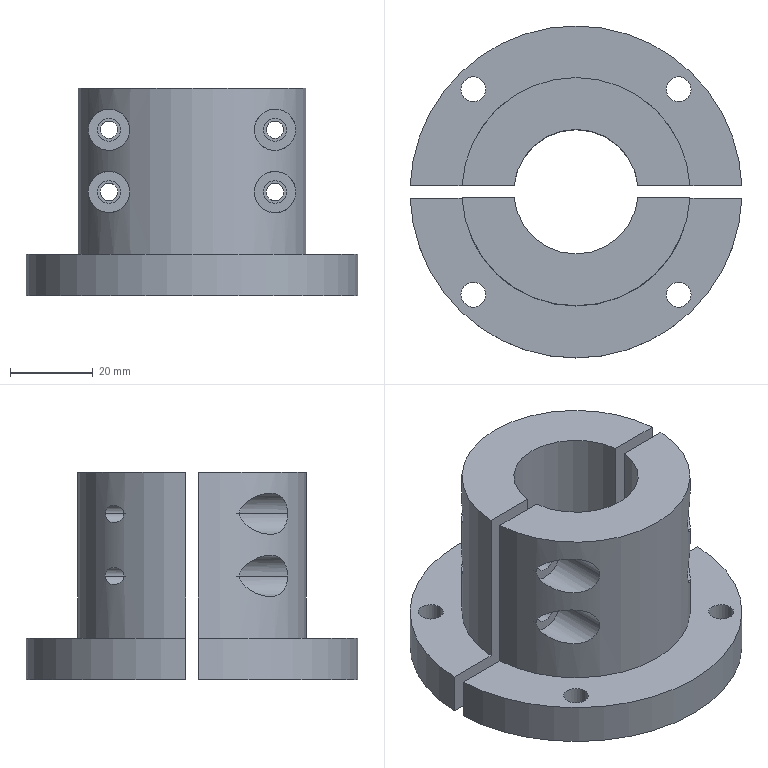NC program | NX | posted with a generic post | part box 79.944 x 80 x 50 mm
Whole program:
N10 G17 G21 G94 G90
(HOLE_MILLING_1 , TOOL : D3)
N12 T17 M6
N14 G54
N16 G17 G0 G90 X-20. Y-15. B0. C0. S9500 M3
N18 G43 Z68.5 H17
N20 Z20.377
N22 G94 G3 X-19.7 Y-15.3 R0.3 F1250.
N24 X-19.4 Y-15. R0.3
N26 X-19.4 Y-15. Z20.177 I-0.6 J0.
N28 X-19.4 Y-15. Z19.977 I-0.6 J0.
N30 X-19.4 Y-15. Z19.777 I-0.6 J0.
N32 X-19.4 Y-15. Z19.577 I-0.6 J0.
N34 X-19.4 Y-15. Z19.377 I-0.6 J0.
N36 X-19.4 Y-15. Z19.177 I-0.6 J0.
N38 X-19.4 Y-15. Z18.977 I-0.6 J0.
N40 X-19.4 Y-15. Z18.777 I-0.6 J0.
N42 X-19.4 Y-15. Z18.577 I-0.6 J0.
N44 X-19.4 Y-15. Z18.377 I-0.6 J0.
N46 X-19.4 Y-15. Z18.177 I-0.6 J0.
N48 X-19.4 Y-15. Z17.977 I-0.6 J0.
N50 X-19.4 Y-15. Z17.777 I-0.6 J0.
N52 X-19.4 Y-15. Z17.577 I-0.6 J0.
N54 X-19.4 Y-15. Z17.377 I-0.6 J0.
N56 X-19.4 Y-15. Z17.177 I-0.6 J0.
N58 X-19.4 Y-15. Z16.977 I-0.6 J0.
N60 X-19.4 Y-15. Z16.777 I-0.6 J0.
N62 X-19.4 Y-15. Z16.577 I-0.6 J0.
N64 X-19.4 Y-15. Z16.377 I-0.6 J0.
N66 X-19.4 Y-15. Z16.177 I-0.6 J0.
N68 X-19.4 Y-15. Z15.977 I-0.6 J0.
N70 X-19.4 Y-15. Z15.777 I-0.6 J0.
N72 X-19.4 Y-15. Z15.577 I-0.6 J0.
N74 X-19.4 Y-15. Z15.377 I-0.6 J0.
N76 X-19.4 Y-15. Z15.177 I-0.6 J0.
N78 X-19.4 Y-15. Z14.977 I-0.6 J0.
N80 X-19.4 Y-15. Z14.777 I-0.6 J0.
N82 X-19.4 Y-15. Z14.577 I-0.6 J0.
N84 X-19.4 Y-15. Z14.377 I-0.6 J0.
N86 X-20. Y-14.4 R0.6
N88 X-19.4 Y-15. R-0.6
N90 X-19.7 Y-14.7 R0.3
N92 X-20. Y-15. R0.3
N94 G0 Z68.5
N96 Y0.
N98 Z20.377
N100 G3 X-19.7 Y-0.3 R0.3
N102 X-19.4 Y0. R0.3
N104 X-19.4 Y0. Z20.177 I-0.6 J0.
N106 X-19.4 Y0. Z19.977 I-0.6 J0.
N108 X-19.4 Y0. Z19.777 I-0.6 J0.
N110 X-19.4 Y0. Z19.577 I-0.6 J0.
N112 X-19.4 Y0. Z19.377 I-0.6 J0.
N114 X-19.4 Y0. Z19.177 I-0.6 J0.
N116 X-19.4 Y0. Z18.977 I-0.6 J0.
N118 X-19.4 Y0. Z18.777 I-0.6 J0.
N120 X-19.4 Y0. Z18.577 I-0.6 J0.
N122 X-19.4 Y0. Z18.377 I-0.6 J0.
N124 X-19.4 Y0. Z18.177 I-0.6 J0.
N126 X-19.4 Y0. Z17.977 I-0.6 J0.
N128 X-19.4 Y0. Z17.777 I-0.6 J0.
N130 X-19.4 Y0. Z17.577 I-0.6 J0.
N132 X-19.4 Y0. Z17.377 I-0.6 J0.
N134 X-19.4 Y0. Z17.177 I-0.6 J0.
N136 X-19.4 Y0. Z16.977 I-0.6 J0.
N138 X-19.4 Y0. Z16.777 I-0.6 J0.
N140 X-19.4 Y0. Z16.577 I-0.6 J0.
N142 X-19.4 Y0. Z16.377 I-0.6 J0.
N144 X-19.4 Y0. Z16.177 I-0.6 J0.
N146 X-19.4 Y0. Z15.977 I-0.6 J0.
N148 X-19.4 Y0. Z15.777 I-0.6 J0.
N150 X-19.4 Y0. Z15.577 I-0.6 J0.
N152 X-19.4 Y0. Z15.377 I-0.6 J0.
N154 X-19.4 Y0. Z15.177 I-0.6 J0.
N156 X-19.4 Y0. Z14.977 I-0.6 J0.
N158 X-19.4 Y0. Z14.777 I-0.6 J0.
N160 X-19.4 Y0. Z14.577 I-0.6 J0.
N162 X-19.4 Y0. Z14.377 I-0.6 J0.
N164 X-20. Y0.6 R0.6
N166 X-19.4 Y0. R-0.6
N168 X-19.7 Y0.3 R0.3
N170 X-20. Y0. R0.3
N172 G0 Z68.5
N174 X20.
N176 Z20.377
N178 G3 X20.3 Y-0.3 R0.3
N180 X20.6 Y0. R0.3
N182 X20.6 Y0. Z20.177 I-0.6 J0.
N184 X20.6 Y0. Z19.977 I-0.6 J0.
N186 X20.6 Y0. Z19.777 I-0.6 J0.
N188 X20.6 Y0. Z19.577 I-0.6 J0.
N190 X20.6 Y0. Z19.377 I-0.6 J0.
N192 X20.6 Y0. Z19.177 I-0.6 J0.
N194 X20.6 Y0. Z18.977 I-0.6 J0.
N196 X20.6 Y0. Z18.777 I-0.6 J0.
N198 X20.6 Y0. Z18.577 I-0.6 J0.
N200 X20.6 Y0. Z18.377 I-0.6 J0.
N202 X20.6 Y0. Z18.177 I-0.6 J0.
N204 X20.6 Y0. Z17.977 I-0.6 J0.
N206 X20.6 Y0. Z17.777 I-0.6 J0.
N208 X20.6 Y0. Z17.577 I-0.6 J0.
N210 X20.6 Y0. Z17.377 I-0.6 J0.
N212 X20.6 Y0. Z17.177 I-0.6 J0.
N214 X20.6 Y0. Z16.977 I-0.6 J0.
N216 X20.6 Y0. Z16.777 I-0.6 J0.
N218 X20.6 Y0. Z16.577 I-0.6 J0.
N220 X20.6 Y0. Z16.377 I-0.6 J0.
N222 X20.6 Y0. Z16.177 I-0.6 J0.
N224 X20.6 Y0. Z15.977 I-0.6 J0.
N226 X20.6 Y0. Z15.777 I-0.6 J0.
N228 X20.6 Y0. Z15.577 I-0.6 J0.
N230 X20.6 Y0. Z15.377 I-0.6 J0.
N232 X20.6 Y0. Z15.177 I-0.6 J0.
N234 X20.6 Y0. Z14.977 I-0.6 J0.
N236 X20.6 Y0. Z14.777 I-0.6 J0.
N238 X20.6 Y0. Z14.577 I-0.6 J0.
N240 X20.6 Y0. Z14.377 I-0.6 J0.
N242 X20. Y0.6 R0.6
N244 X20.6 Y0. R-0.6
N246 X20.3 Y0.3 R0.3
N248 X20. Y0. R0.3
N250 G0 Z68.5
N252 Y-15.
N254 Z20.377
N256 G3 X20.3 Y-15.3 R0.3
N258 X20.6 Y-15. R0.3
N260 X20.6 Y-15. Z20.177 I-0.6 J0.
N262 X20.6 Y-15. Z19.977 I-0.6 J0.
N264 X20.6 Y-15. Z19.777 I-0.6 J0.
N266 X20.6 Y-15. Z19.577 I-0.6 J0.
N268 X20.6 Y-15. Z19.377 I-0.6 J0.
N270 X20.6 Y-15. Z19.177 I-0.6 J0.
N272 X20.6 Y-15. Z18.977 I-0.6 J0.
N274 X20.6 Y-15. Z18.777 I-0.6 J0.
N276 X20.6 Y-15. Z18.577 I-0.6 J0.
N278 X20.6 Y-15. Z18.377 I-0.6 J0.
N280 X20.6 Y-15. Z18.177 I-0.6 J0.
N282 X20.6 Y-15. Z17.977 I-0.6 J0.
N284 X20.6 Y-15. Z17.777 I-0.6 J0.
N286 X20.6 Y-15. Z17.577 I-0.6 J0.
N288 X20.6 Y-15. Z17.377 I-0.6 J0.
N290 X20.6 Y-15. Z17.177 I-0.6 J0.
N292 X20.6 Y-15. Z16.977 I-0.6 J0.
N294 X20.6 Y-15. Z16.777 I-0.6 J0.
N296 X20.6 Y-15. Z16.577 I-0.6 J0.
N298 X20.6 Y-15. Z16.377 I-0.6 J0.
N300 X20.6 Y-15. Z16.177 I-0.6 J0.
N302 X20.6 Y-15. Z15.977 I-0.6 J0.
N304 X20.6 Y-15. Z15.777 I-0.6 J0.
N306 X20.6 Y-15. Z15.577 I-0.6 J0.
N308 X20.6 Y-15. Z15.377 I-0.6 J0.
N310 X20.6 Y-15. Z15.177 I-0.6 J0.
N312 X20.6 Y-15. Z14.977 I-0.6 J0.
N314 X20.6 Y-15. Z14.777 I-0.6 J0.
N316 X20.6 Y-15. Z14.577 I-0.6 J0.
N318 X20.6 Y-15. Z14.377 I-0.6 J0.
N320 X20. Y-14.4 R0.6
N322 X20.6 Y-15. R-0.6
N324 X20.3 Y-14.7 R0.3
N326 X20. Y-15. R0.3
N328 G0 Z68.5
N330 M5
(DRILLING_COPY_1_COPY_1 , TOOL : D4A45)
N332 T18 M6
N334 G54
N336 G17 G0 G90 X-20. Y0. B0. C0. S5000 M3
N338 G43 Z68.5 H18
N340 G94 G81 G98 Z13.377 F350. R17.377
N342 Y-15.
N344 X20.
N346 Y0.
N348 G80
N350 G0 X20. Y0. Z68.5
N352 M5
(DRILLING_COPY_1_COPY_COPY_1 , TOOL : 4.2ZT)
N354 T04 M6
N356 G54
N358 G17 G0 G90 X-20. Y0. B0. C0. S2000 M3
N360 G43 Z68.5 H4
N362 G94 G83 G98 Z-2.762 F200. Q2. R22.377
N364 Y-15.
N366 X20.
N368 Y0.
N370 G80
N372 G0 X20. Y0. Z68.5
N374 M5
N376 M2